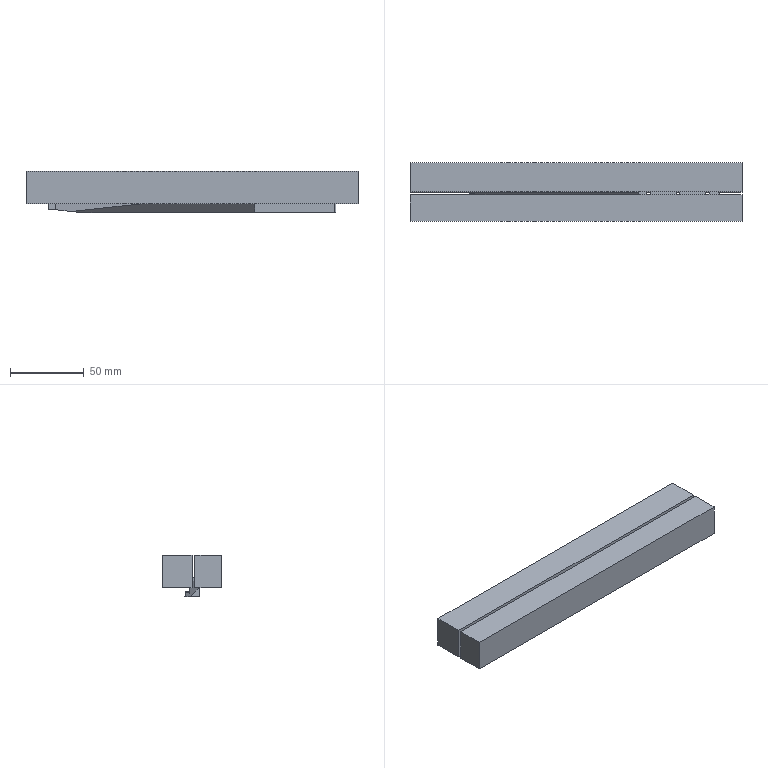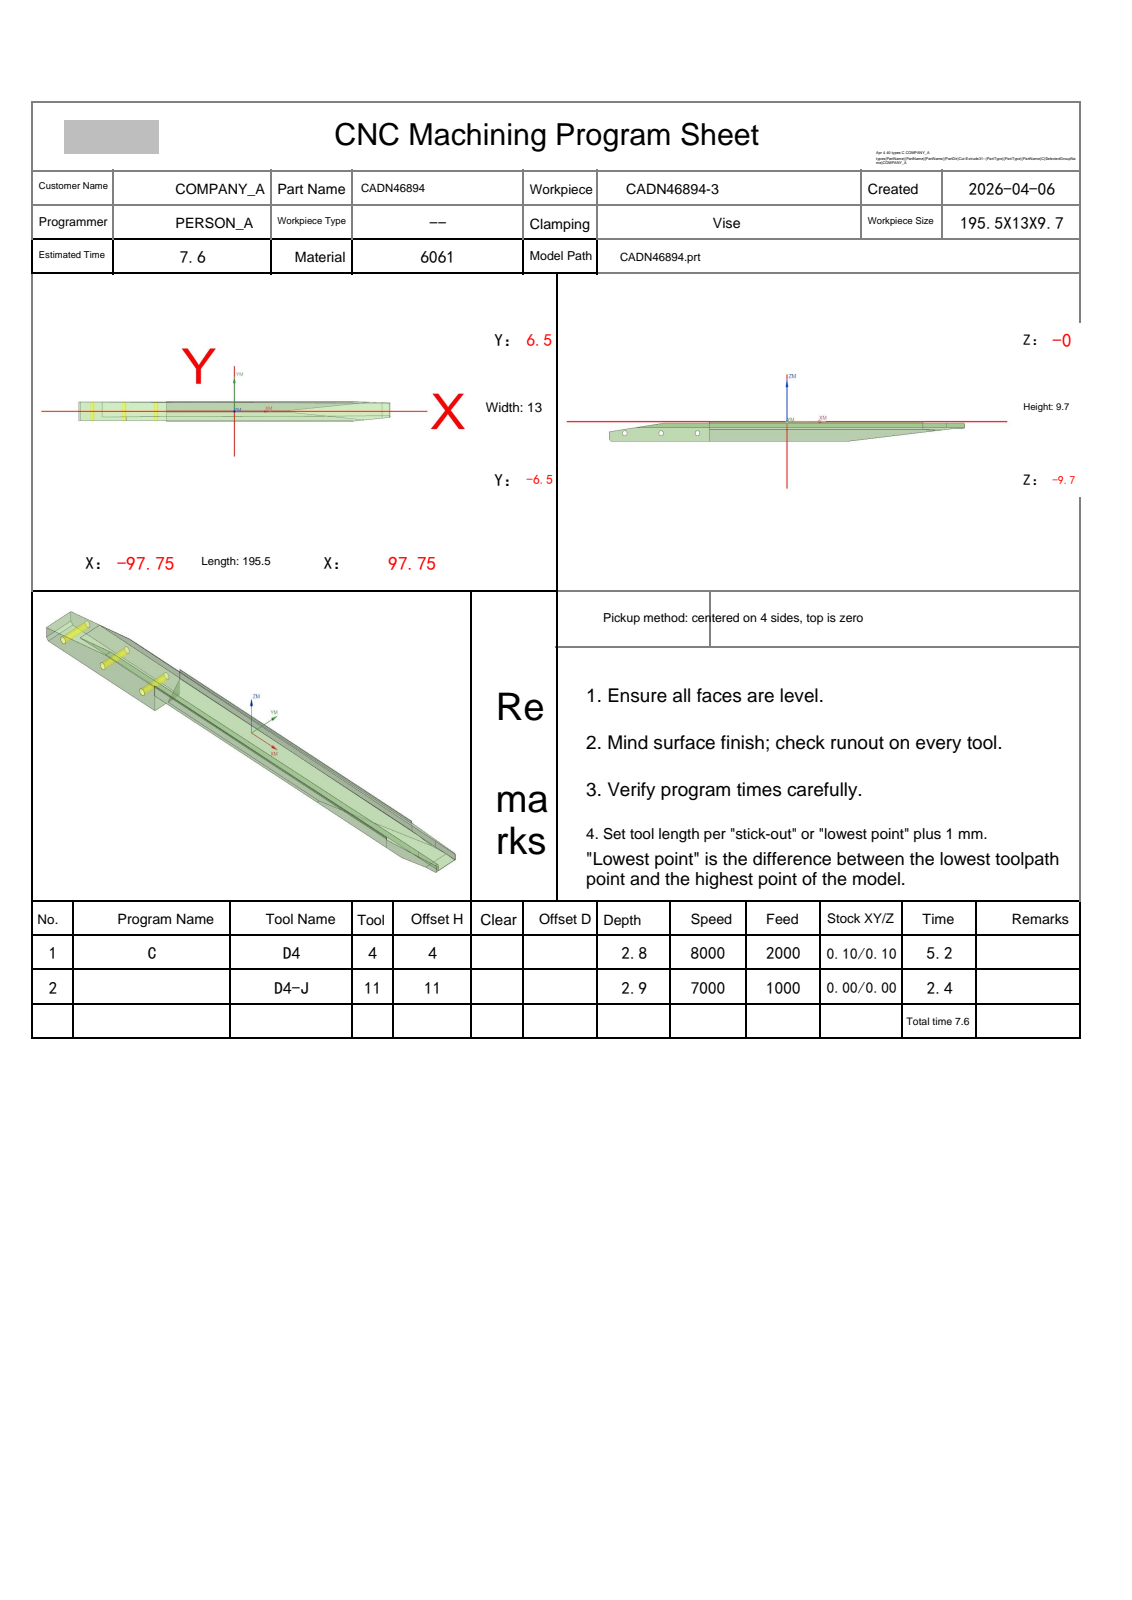NC program | NX | posted by the shop | part box 225.5 x 39.7 x 28 mm
Lines 1 to 1334 of 20119:
%
O0001
(Machine time: 20.00 MIN)
(===Total Tool:4===)
(T4=D4      D=4.   R=0.   D-  H04 Z=-12.35)
(T17=D2-J   D=2.   R=0.   D-  H17 Z=-12.4 )
(T19=D1.5-J D=1.5  R=0.   D-  H19 Z=-12.4 )
(T2=D6 chamfer tool   D=6.   R=0.   D-  H02 Z=-7.2  )
G80 G90 G17 G49 G40
G91 G28 Z0
M01
N1 T04 M06
(D4  D=4. R=0. H=04 ce=0.05 di=0.05)
G00 G90 G54 X-83.137 Y-4.487 M03 S8000
G43 H04 Z44.
M08
Z-5.5
G01 X-109.809 Y-4.336 Z-6.199 F2000.
X-142.722 Y-4.15
X-163.733 Y-4.85
X-163.768
G02 X-165.219 Y-4.641 I0.0 J5.15
X-166.626 Y-5.054 I-2.137 J4.685
G01 X-170.088 Y-5.55
X-65.732
G02 X-64.212 Y-5.779 I0.0 J-5.15
X-62.726 Y-5.387 I2.042 J-4.728
G01 X-55.848 Y-4.641
X-53.937 Y-4.05
X-49.469
X-53.851 Y-4.525
G03 X-53.937 Y-4.05 I-1.997 J-.116
G01 X-55.848 Y-4.641
X-109.809 Y-4.336
X-109.796 Y-2.05
X-142.751
X-143.451 Y-2.75
X-163.768
G02 X-165.387 Y-2.285 I0.0 J3.05
X-166.924 Y-2.975 I-1.969 J2.329
G01 X-193.45 Y-6.777
Y-7.725
G02 X-192.5 Y-7.65 I.95 J-5.975
G01 X-65.732
G02 X-64.085 Y-8.133 I0.0 J-3.05
X-62.499 Y-7.475 I1.915 J-2.374
G01 X-37.837 Y-4.8
X-21.345
X-21.441 Y-3.021
X-18.939 Y-2.75
X-20.049
X-20.749 Y-2.05
X-109.796
X-110.296
Z-5.699
G00 Z-5.5
X-83.137 Y-4.487
Z-5.699
G01 X-109.809 Y-4.336 Z-6.397
X-142.722 Y-4.15
X-163.733 Y-4.85
X-163.768
G02 X-165.219 Y-4.641 I0.0 J5.15
X-166.626 Y-5.054 I-2.137 J4.685
G01 X-170.088 Y-5.55
X-65.732
G02 X-64.212 Y-5.779 I0.0 J-5.15
X-62.726 Y-5.387 I2.042 J-4.728
G01 X-55.848 Y-4.641
X-53.937 Y-4.05
X-49.469
X-53.851 Y-4.525
G03 X-53.937 Y-4.05 I-1.997 J-.116
G01 X-55.848 Y-4.641
X-109.809 Y-4.336
X-109.796 Y-2.05
X-142.751
X-143.451 Y-2.75
X-163.768
G02 X-165.387 Y-2.285 I0.0 J3.05
X-166.924 Y-2.975 I-1.969 J2.329
G01 X-193.45 Y-6.777
Y-7.725
G02 X-192.5 Y-7.65 I.95 J-5.975
G01 X-65.732
G02 X-64.085 Y-8.133 I0.0 J-3.05
X-62.499 Y-7.475 I1.915 J-2.374
G01 X-37.837 Y-4.8
X-21.345
X-21.441 Y-3.021
X-18.939 Y-2.75
X-20.049
X-20.749 Y-2.05
X-109.796
X-110.296
Z-5.897
G00 Z-5.699
X-83.137 Y-4.487
Z-5.897
G01 X-109.809 Y-4.336 Z-6.595
X-142.722 Y-4.15
X-163.733 Y-4.85
X-163.768
G02 X-165.219 Y-4.641 I0.0 J5.15
X-166.626 Y-5.054 I-2.137 J4.685
G01 X-170.088 Y-5.55
X-65.732
G02 X-64.212 Y-5.779 I0.0 J-5.15
X-62.726 Y-5.387 I2.042 J-4.728
G01 X-55.848 Y-4.641
X-53.937 Y-4.05
X-49.469
X-53.851 Y-4.525
G03 X-53.937 Y-4.05 I-1.997 J-.116
G01 X-55.848 Y-4.641
X-109.809 Y-4.336
X-109.796 Y-2.05
X-142.751
X-143.451 Y-2.75
X-163.768
G02 X-165.387 Y-2.285 I0.0 J3.05
X-166.924 Y-2.975 I-1.969 J2.329
G01 X-193.45 Y-6.777
Y-7.725
G02 X-192.5 Y-7.65 I.95 J-5.975
G01 X-65.732
G02 X-64.085 Y-8.133 I0.0 J-3.05
X-62.499 Y-7.475 I1.915 J-2.374
G01 X-37.837 Y-4.8
X-21.345
X-21.441 Y-3.021
X-18.939 Y-2.75
X-20.049
X-20.749 Y-2.05
X-109.796
X-110.296
Z-6.095
G00 Z-5.897
X-83.137 Y-4.487
Z-6.095
G01 X-109.809 Y-4.336 Z-6.794
X-142.722 Y-4.15
X-163.733 Y-4.85
X-163.768
G02 X-165.219 Y-4.641 I0.0 J5.15
X-166.626 Y-5.054 I-2.137 J4.685
G01 X-170.088 Y-5.55
X-65.732
G02 X-64.212 Y-5.779 I0.0 J-5.15
X-62.726 Y-5.387 I2.042 J-4.728
G01 X-55.848 Y-4.641
X-53.937 Y-4.05
X-49.469
X-53.851 Y-4.525
G03 X-53.937 Y-4.05 I-1.997 J-.116
G01 X-55.848 Y-4.641
X-109.809 Y-4.336
X-109.796 Y-2.05
X-142.751
X-143.451 Y-2.75
X-163.768
G02 X-165.387 Y-2.285 I0.0 J3.05
X-166.924 Y-2.975 I-1.969 J2.329
G01 X-193.45 Y-6.777
Y-7.725
G02 X-192.5 Y-7.65 I.95 J-5.975
G01 X-65.732
G02 X-64.085 Y-8.133 I0.0 J-3.05
X-62.499 Y-7.475 I1.915 J-2.374
G01 X-37.837 Y-4.8
X-21.345
X-21.441 Y-3.021
X-18.939 Y-2.75
X-20.049
X-20.749 Y-2.05
X-109.796
X-110.296
Z-6.294
G00 Z-6.095
X-83.137 Y-4.487
Z-6.294
G01 X-109.809 Y-4.336 Z-6.992
X-142.722 Y-4.15
X-163.733 Y-4.85
X-163.768
G02 X-165.219 Y-4.641 I0.0 J5.15
X-166.626 Y-5.054 I-2.137 J4.685
G01 X-170.088 Y-5.55
X-65.732
G02 X-64.212 Y-5.779 I0.0 J-5.15
X-62.726 Y-5.387 I2.042 J-4.728
G01 X-55.848 Y-4.641
X-53.937 Y-4.05
X-49.469
X-53.851 Y-4.525
G03 X-53.937 Y-4.05 I-1.997 J-.116
G01 X-55.848 Y-4.641
X-109.809 Y-4.336
X-109.796 Y-2.05
X-142.751
X-143.451 Y-2.75
X-163.768
G02 X-165.387 Y-2.285 I0.0 J3.05
X-166.924 Y-2.975 I-1.969 J2.329
G01 X-193.45 Y-6.777
Y-7.725
G02 X-192.5 Y-7.65 I.95 J-5.975
G01 X-65.732
G02 X-64.085 Y-8.133 I0.0 J-3.05
X-62.499 Y-7.475 I1.915 J-2.374
G01 X-37.837 Y-4.8
X-21.345
X-21.441 Y-3.021
X-18.939 Y-2.75
X-20.049
X-20.749 Y-2.05
X-109.796
X-110.296
Z-6.492
G00 Z-6.294
X-83.137 Y-4.487
Z-6.492
G01 X-109.809 Y-4.336 Z-7.191
X-142.722 Y-4.15
X-163.733 Y-4.85
X-163.768
G02 X-165.219 Y-4.641 I0.0 J5.15
X-166.626 Y-5.054 I-2.137 J4.685
G01 X-170.088 Y-5.55
X-65.732
G02 X-64.212 Y-5.779 I0.0 J-5.15
X-62.726 Y-5.387 I2.042 J-4.728
G01 X-55.848 Y-4.641
X-53.937 Y-4.05
X-49.469
X-53.851 Y-4.525
G03 X-53.937 Y-4.05 I-1.997 J-.116
G01 X-55.848 Y-4.641
X-109.809 Y-4.336
X-109.796 Y-2.05
X-142.751
X-143.451 Y-2.75
X-163.768
G02 X-165.387 Y-2.285 I0.0 J3.05
X-166.924 Y-2.975 I-1.969 J2.329
G01 X-193.45 Y-6.777
Y-7.725
G02 X-192.5 Y-7.65 I.95 J-5.975
G01 X-65.732
G02 X-64.085 Y-8.133 I0.0 J-3.05
X-62.499 Y-7.475 I1.915 J-2.374
G01 X-37.837 Y-4.8
X-21.345
X-21.441 Y-3.021
X-18.939 Y-2.75
X-20.049
X-20.749 Y-2.05
X-109.796
X-110.296
Z-6.691
G00 Z-6.492
X-83.137 Y-4.487
Z-6.691
G01 X-109.809 Y-4.336 Z-7.389
X-142.722 Y-4.15
X-163.733 Y-4.85
X-163.768
G02 X-165.219 Y-4.641 I0.0 J5.15
X-166.626 Y-5.054 I-2.137 J4.685
G01 X-170.088 Y-5.55
X-65.732
G02 X-64.212 Y-5.779 I0.0 J-5.15
X-62.726 Y-5.387 I2.042 J-4.728
G01 X-55.848 Y-4.641
X-53.937 Y-4.05
X-49.469
X-53.851 Y-4.525
G03 X-53.937 Y-4.05 I-1.997 J-.116
G01 X-55.848 Y-4.641
X-109.809 Y-4.336
X-109.796 Y-2.05
X-142.751
X-143.451 Y-2.75
X-163.768
G02 X-165.387 Y-2.285 I0.0 J3.05
X-166.924 Y-2.975 I-1.969 J2.329
G01 X-193.45 Y-6.777
Y-7.725
G02 X-192.5 Y-7.65 I.95 J-5.975
G01 X-65.732
G02 X-64.085 Y-8.133 I0.0 J-3.05
X-62.499 Y-7.475 I1.915 J-2.374
G01 X-37.837 Y-4.8
X-21.345
X-21.441 Y-3.021
X-18.939 Y-2.75
X-20.049
X-20.749 Y-2.05
X-109.796
X-110.296
Z-6.889
G00 Z-6.691
X-83.137 Y-4.487
Z-6.889
G01 X-109.809 Y-4.336 Z-7.588
X-142.722 Y-4.15
X-163.733 Y-4.85
X-163.768
G02 X-165.219 Y-4.641 I0.0 J5.15
X-166.626 Y-5.054 I-2.137 J4.685
G01 X-170.088 Y-5.55
X-65.732
G02 X-64.212 Y-5.779 I0.0 J-5.15
X-62.726 Y-5.387 I2.042 J-4.728
G01 X-55.848 Y-4.641
X-53.937 Y-4.05
X-49.469
X-53.851 Y-4.525
G03 X-53.937 Y-4.05 I-1.997 J-.116
G01 X-55.848 Y-4.641
X-109.809 Y-4.336
X-109.796 Y-2.05
X-142.751
X-143.451 Y-2.75
X-163.768
G02 X-165.387 Y-2.285 I0.0 J3.05
X-166.924 Y-2.975 I-1.969 J2.329
G01 X-193.45 Y-6.777
Y-7.725
G02 X-192.5 Y-7.65 I.95 J-5.975
G01 X-65.732
G02 X-64.085 Y-8.133 I0.0 J-3.05
X-62.499 Y-7.475 I1.915 J-2.374
G01 X-37.837 Y-4.8
X-21.345
X-21.441 Y-3.021
X-18.939 Y-2.75
X-20.049
X-20.749 Y-2.05
X-109.796
X-110.296
Z-7.088
G00 Z-6.889
X-83.137 Y-4.487
Z-7.088
G01 X-109.809 Y-4.336 Z-7.786
X-142.722 Y-4.15
X-163.733 Y-4.85
X-163.768
G02 X-165.219 Y-4.641 I0.0 J5.15
X-166.626 Y-5.054 I-2.137 J4.685
G01 X-170.088 Y-5.55
X-65.732
G02 X-64.212 Y-5.779 I0.0 J-5.15
X-62.726 Y-5.387 I2.042 J-4.728
G01 X-55.848 Y-4.641
X-53.937 Y-4.05
X-49.469
X-53.851 Y-4.525
G03 X-53.937 Y-4.05 I-1.997 J-.116
G01 X-55.848 Y-4.641
X-109.809 Y-4.336
X-109.796 Y-2.05
X-142.751
X-143.451 Y-2.75
X-163.768
G02 X-165.387 Y-2.285 I0.0 J3.05
X-166.924 Y-2.975 I-1.969 J2.329
G01 X-193.45 Y-6.777
Y-7.725
G02 X-192.5 Y-7.65 I.95 J-5.975
G01 X-65.732
G02 X-64.085 Y-8.133 I0.0 J-3.05
X-62.499 Y-7.475 I1.915 J-2.374
G01 X-37.837 Y-4.8
X-21.345
X-21.441 Y-3.021
X-18.939 Y-2.75
X-20.049
X-20.749 Y-2.05
X-109.796
X-110.296
Z-7.286
G00 Z-7.088
X-83.137 Y-4.487
Z-7.286
G01 X-109.809 Y-4.336 Z-7.984
X-142.722 Y-4.15
X-163.733 Y-4.85
X-163.768
G02 X-165.219 Y-4.641 I0.0 J5.15
X-166.626 Y-5.054 I-2.137 J4.685
G01 X-170.088 Y-5.55
X-65.732
G02 X-64.212 Y-5.779 I0.0 J-5.15
X-62.726 Y-5.387 I2.042 J-4.728
G01 X-55.848 Y-4.641
X-53.937 Y-4.05
X-49.469
X-53.851 Y-4.525
G03 X-53.937 Y-4.05 I-1.997 J-.116
G01 X-55.848 Y-4.641
X-109.809 Y-4.336
X-109.796 Y-2.05
X-142.751
X-143.451 Y-2.75
X-163.768
G02 X-165.387 Y-2.285 I0.0 J3.05
X-166.924 Y-2.975 I-1.969 J2.329
G01 X-193.45 Y-6.777
Y-7.725
G02 X-192.5 Y-7.65 I.95 J-5.975
G01 X-65.732
G02 X-64.085 Y-8.133 I0.0 J-3.05
X-62.499 Y-7.475 I1.915 J-2.374
G01 X-37.837 Y-4.8
X-21.345
X-21.441 Y-3.021
X-18.939 Y-2.75
X-20.049
X-20.749 Y-2.05
X-109.796
X-110.296
Z-7.484
G00 Z-7.286
X-83.137 Y-4.487
Z-7.484
G01 X-109.809 Y-4.336 Z-8.183
X-142.722 Y-4.15
X-163.733 Y-4.85
X-163.768
G02 X-165.219 Y-4.641 I0.0 J5.15
X-166.626 Y-5.054 I-2.137 J4.685
G01 X-170.088 Y-5.55
X-65.732
G02 X-64.212 Y-5.779 I0.0 J-5.15
X-62.726 Y-5.387 I2.042 J-4.728
G01 X-55.848 Y-4.641
X-53.937 Y-4.05
X-49.469
X-53.851 Y-4.525
G03 X-53.937 Y-4.05 I-1.997 J-.116
G01 X-55.848 Y-4.641
X-109.809 Y-4.336
X-109.796 Y-2.05
X-142.751
X-143.451 Y-2.75
X-163.768
G02 X-165.387 Y-2.285 I0.0 J3.05
X-166.924 Y-2.975 I-1.969 J2.329
G01 X-193.45 Y-6.777
Y-7.725
G02 X-192.5 Y-7.65 I.95 J-5.975
G01 X-65.732
G02 X-64.085 Y-8.133 I0.0 J-3.05
X-62.499 Y-7.475 I1.915 J-2.374
G01 X-37.837 Y-4.8
X-21.345
X-21.441 Y-3.021
X-18.939 Y-2.75
X-20.049
X-20.749 Y-2.05
X-109.796
X-110.296
Z-7.683
G00 Z-7.484
X-83.137 Y-4.487
Z-7.683
G01 X-109.809 Y-4.336 Z-8.381
X-142.722 Y-4.15
X-163.733 Y-4.85
X-163.768
G02 X-165.219 Y-4.641 I0.0 J5.15
X-166.626 Y-5.054 I-2.137 J4.685
G01 X-170.088 Y-5.55
X-65.732
G02 X-64.212 Y-5.779 I0.0 J-5.15
X-62.726 Y-5.387 I2.042 J-4.728
G01 X-55.848 Y-4.641
X-53.937 Y-4.05
X-49.469
X-53.851 Y-4.525
G03 X-53.937 Y-4.05 I-1.997 J-.116
G01 X-55.848 Y-4.641
X-109.809 Y-4.336
X-109.796 Y-2.05
X-142.751
X-143.451 Y-2.75
X-163.768
G02 X-165.387 Y-2.285 I0.0 J3.05
X-166.924 Y-2.975 I-1.969 J2.329
G01 X-193.45 Y-6.777
Y-7.725
G02 X-192.5 Y-7.65 I.95 J-5.975
G01 X-65.732
G02 X-64.085 Y-8.133 I0.0 J-3.05
X-62.499 Y-7.475 I1.915 J-2.374
G01 X-37.837 Y-4.8
X-21.345
X-21.441 Y-3.021
X-18.939 Y-2.75
X-20.049
X-20.749 Y-2.05
X-109.796
X-110.296
Z-7.881
G00 Z-7.683
X-83.137 Y-4.487
Z-7.881
G01 X-109.809 Y-4.336 Z-8.58
X-142.722 Y-4.15
X-163.733 Y-4.85
X-163.768
G02 X-165.219 Y-4.641 I0.0 J5.15
X-166.626 Y-5.054 I-2.137 J4.685
G01 X-170.088 Y-5.55
X-65.732
G02 X-64.212 Y-5.779 I0.0 J-5.15
X-62.726 Y-5.387 I2.042 J-4.728
G01 X-55.848 Y-4.641
X-53.937 Y-4.05
X-49.469
X-53.851 Y-4.525
G03 X-53.937 Y-4.05 I-1.997 J-.116
G01 X-55.848 Y-4.641
X-109.809 Y-4.336
X-109.796 Y-2.05
X-142.751
X-143.451 Y-2.75
X-163.768
G02 X-165.387 Y-2.285 I0.0 J3.05
X-166.924 Y-2.975 I-1.969 J2.329
G01 X-193.45 Y-6.777
Y-7.725
G02 X-192.5 Y-7.65 I.95 J-5.975
G01 X-65.732
G02 X-64.085 Y-8.133 I0.0 J-3.05
X-62.499 Y-7.475 I1.915 J-2.374
G01 X-37.837 Y-4.8
X-21.345
X-21.441 Y-3.021
X-18.939 Y-2.75
X-20.049
X-20.749 Y-2.05
X-109.796
X-110.296
Z-8.08
G00 Z-7.881
X-83.137 Y-4.487
Z-8.08
G01 X-109.809 Y-4.336 Z-8.778
X-142.722 Y-4.15
X-163.733 Y-4.85
X-163.768
G02 X-165.219 Y-4.641 I0.0 J5.15
X-166.626 Y-5.054 I-2.137 J4.685
G01 X-170.088 Y-5.55
X-65.732
G02 X-64.212 Y-5.779 I0.0 J-5.15
X-62.726 Y-5.387 I2.042 J-4.728
G01 X-55.848 Y-4.641
X-53.937 Y-4.05
X-49.469
X-53.851 Y-4.525
G03 X-53.937 Y-4.05 I-1.997 J-.116
G01 X-55.848 Y-4.641
X-109.809 Y-4.336
X-109.796 Y-2.05
X-142.751
X-143.451 Y-2.75
X-163.768
G02 X-165.387 Y-2.285 I0.0 J3.05
X-166.924 Y-2.975 I-1.969 J2.329
G01 X-193.45 Y-6.777
Y-7.725
G02 X-192.5 Y-7.65 I.95 J-5.975
G01 X-65.732
G02 X-64.085 Y-8.133 I0.0 J-3.05
X-62.499 Y-7.475 I1.915 J-2.374
G01 X-37.837 Y-4.8
X-21.345
X-21.441 Y-3.021
X-18.939 Y-2.75
X-20.049
X-20.749 Y-2.05
X-109.796
X-110.296
Z-8.278
G00 Z-8.08
X-83.137 Y-4.487
Z-8.278
G01 X-109.809 Y-4.336 Z-8.977
X-142.722 Y-4.15
X-163.733 Y-4.85
X-163.768
G02 X-165.219 Y-4.641 I0.0 J5.15
X-166.626 Y-5.054 I-2.137 J4.685
G01 X-170.088 Y-5.55
X-65.732
G02 X-64.212 Y-5.779 I0.0 J-5.15
X-62.726 Y-5.387 I2.042 J-4.728
G01 X-55.848 Y-4.641
X-53.937 Y-4.05
X-49.469
X-53.851 Y-4.525
G03 X-53.937 Y-4.05 I-1.997 J-.116
G01 X-55.848 Y-4.641
X-109.809 Y-4.336
X-109.796 Y-2.05
X-142.751
X-143.451 Y-2.75
X-163.768
G02 X-165.387 Y-2.285 I0.0 J3.05
X-166.924 Y-2.975 I-1.969 J2.329
G01 X-193.45 Y-6.777
Y-7.725
G02 X-192.5 Y-7.65 I.95 J-5.975
G01 X-65.732
G02 X-64.085 Y-8.133 I0.0 J-3.05
X-62.499 Y-7.475 I1.915 J-2.374
G01 X-37.837 Y-4.8
X-21.345
X-21.441 Y-3.021
X-18.939 Y-2.75
X-20.049
X-20.749 Y-2.05
X-109.796
X-110.296
Z-8.477
G00 Z-8.278
X-83.137 Y-4.487
Z-8.477
G01 X-109.809 Y-4.336 Z-9.175
X-142.722 Y-4.15
X-163.733 Y-4.85
X-163.768
G02 X-165.219 Y-4.641 I0.0 J5.15
X-166.626 Y-5.054 I-2.137 J4.685
G01 X-170.088 Y-5.55
X-65.732
G02 X-64.212 Y-5.779 I0.0 J-5.15
X-62.726 Y-5.387 I2.042 J-4.728
G01 X-55.848 Y-4.641
X-53.937 Y-4.05
X-49.469
X-53.851 Y-4.525
G03 X-53.937 Y-4.05 I-1.997 J-.116
G01 X-55.848 Y-4.641
X-109.809 Y-4.336
X-109.796 Y-2.05
X-142.751
X-143.451 Y-2.75
X-163.768
G02 X-165.387 Y-2.285 I0.0 J3.05
X-166.924 Y-2.975 I-1.969 J2.329
G01 X-193.45 Y-6.777
Y-7.725
G02 X-192.5 Y-7.65 I.95 J-5.975
G01 X-65.732
G02 X-64.085 Y-8.133 I0.0 J-3.05
X-62.499 Y-7.475 I1.915 J-2.374
G01 X-37.837 Y-4.8
X-21.345
X-21.441 Y-3.021
X-18.939 Y-2.75
X-20.049
X-20.749 Y-2.05
X-109.796
X-110.296
Z-8.675
G00 Z-8.477
X-83.137 Y-4.487
Z-8.675
G01 X-109.809 Y-4.336 Z-9.373
X-142.722 Y-4.15
X-163.733 Y-4.85
X-163.768
G02 X-165.219 Y-4.641 I0.0 J5.15
X-166.626 Y-5.054 I-2.137 J4.685
G01 X-170.088 Y-5.55
X-65.732
G02 X-64.212 Y-5.779 I0.0 J-5.15
X-62.726 Y-5.387 I2.042 J-4.728
G01 X-55.848 Y-4.641
X-53.937 Y-4.05
X-49.469
X-53.851 Y-4.525
G03 X-53.937 Y-4.05 I-1.997 J-.116
G01 X-55.848 Y-4.641
X-109.809 Y-4.336
X-109.796 Y-2.05
X-142.751
X-143.451 Y-2.75
X-163.768
G02 X-165.387 Y-2.285 I0.0 J3.05
X-166.924 Y-2.975 I-1.969 J2.329
G01 X-193.45 Y-6.777
Y-7.725
G02 X-192.5 Y-7.65 I.95 J-5.975
G01 X-65.732
G02 X-64.085 Y-8.133 I0.0 J-3.05
X-62.499 Y-7.475 I1.915 J-2.374
G01 X-37.837 Y-4.8
X-21.345
X-21.441 Y-3.021
X-18.939 Y-2.75
X-20.049
X-20.749 Y-2.05
X-109.796
X-110.296
Z-8.873
G00 Z-8.675
X-83.137 Y-4.487
Z-8.873
G01 X-109.809 Y-4.336 Z-9.572
X-142.722 Y-4.15
X-163.733 Y-4.85
X-163.768
G02 X-165.219 Y-4.641 I0.0 J5.15
X-166.626 Y-5.054 I-2.137 J4.685
G01 X-170.088 Y-5.55
X-65.732
G02 X-64.212 Y-5.779 I0.0 J-5.15
X-62.726 Y-5.387 I2.042 J-4.728
G01 X-55.848 Y-4.641
X-53.937 Y-4.05
X-49.469
X-53.851 Y-4.525
G03 X-53.937 Y-4.05 I-1.997 J-.116
G01 X-55.848 Y-4.641
X-109.809 Y-4.336
X-109.796 Y-2.05
X-142.751
X-143.451 Y-2.75
X-163.768
G02 X-165.387 Y-2.285 I0.0 J3.05
X-166.924 Y-2.975 I-1.969 J2.329
G01 X-193.45 Y-6.777
Y-7.725
G02 X-192.5 Y-7.65 I.95 J-5.975
G01 X-65.732
G02 X-64.085 Y-8.133 I0.0 J-3.05
X-62.499 Y-7.475 I1.915 J-2.374
G01 X-37.837 Y-4.8
X-21.345
X-21.441 Y-3.021
X-18.939 Y-2.75
X-20.049
X-20.749 Y-2.05
X-109.796
X-110.296
Z-9.072
G00 Z-8.873
X-83.137 Y-4.487
Z-9.072
G01 X-109.809 Y-4.336 Z-9.77
X-142.722 Y-4.15
X-163.733 Y-4.85
X-163.768
G02 X-165.219 Y-4.641 I0.0 J5.15
X-166.626 Y-5.054 I-2.137 J4.685
G01 X-170.088 Y-5.55
X-65.732
G02 X-64.212 Y-5.779 I0.0 J-5.15
X-62.726 Y-5.387 I2.042 J-4.728
G01 X-55.848 Y-4.641
X-53.937 Y-4.05
X-49.469
X-53.851 Y-4.525
G03 X-53.937 Y-4.05 I-1.997 J-.116
G01 X-55.848 Y-4.641
X-109.809 Y-4.336
X-109.796 Y-2.05
X-142.751
X-143.451 Y-2.75
X-163.768
G02 X-165.387 Y-2.285 I0.0 J3.05
X-166.924 Y-2.975 I-1.969 J2.329
G01 X-193.45 Y-6.777
Y-7.725
G02 X-192.5 Y-7.65 I.95 J-5.975
G01 X-65.732
G02 X-64.085 Y-8.133 I0.0 J-3.05
X-62.499 Y-7.475 I1.915 J-2.374
G01 X-37.837 Y-4.8
X-21.345
X-21.441 Y-3.021
X-18.939 Y-2.75
X-20.049
X-20.749 Y-2.05
X-109.796
X-110.296
Z-9.27
G00 Z-9.072
X-83.137 Y-4.487
Z-9.27
G01 X-109.809 Y-4.336 Z-9.969
X-142.722 Y-4.15
X-163.733 Y-4.85
X-163.768
G02 X-165.219 Y-4.641 I0.0 J5.15
X-166.626 Y-5.054 I-2.137 J4.685
G01 X-170.088 Y-5.55
X-65.732
G02 X-64.212 Y-5.779 I0.0 J-5.15
X-62.726 Y-5.387 I2.042 J-4.728
G01 X-55.848 Y-4.641
X-53.937 Y-4.05
X-49.469
X-53.851 Y-4.525
G03 X-53.937 Y-4.05 I-1.997 J-.116
G01 X-55.848 Y-4.641
X-109.809 Y-4.336
X-109.796 Y-2.05
X-142.751
X-143.451 Y-2.75
X-163.768
G02 X-165.387 Y-2.285 I0.0 J3.05
X-166.924 Y-2.975 I-1.969 J2.329
G01 X-193.45 Y-6.777
Y-7.725
G02 X-192.5 Y-7.65 I.95 J-5.975
G01 X-65.732
G02 X-64.085 Y-8.133 I0.0 J-3.05
X-62.499 Y-7.475 I1.915 J-2.374
G01 X-37.837 Y-4.8
X-21.345
X-21.441 Y-3.021
X-18.939 Y-2.75
X-20.049
X-20.749 Y-2.05
X-109.796
X-110.296
Z-9.469
G00 Z-9.27
X-83.137 Y-4.487
Z-9.469
G01 X-109.809 Y-4.336 Z-10.167
X-142.722 Y-4.15
X-163.733 Y-4.85
X-163.768
G02 X-165.219 Y-4.641 I0.0 J5.15
X-166.626 Y-5.054 I-2.137 J4.685
G01 X-170.088 Y-5.55
X-65.732
G02 X-64.212 Y-5.779 I0.0 J-5.15
X-62.726 Y-5.387 I2.042 J-4.728
G01 X-55.848 Y-4.641
X-53.937 Y-4.05
X-49.469
X-53.851 Y-4.525
G03 X-53.937 Y-4.05 I-1.997 J-.116
G01 X-55.848 Y-4.641
X-109.809 Y-4.336
X-109.796 Y-2.05
X-142.751
X-143.451 Y-2.75
X-163.768
G02 X-165.387 Y-2.285 I0.0 J3.05
X-166.924 Y-2.975 I-1.969 J2.329
G01 X-193.45 Y-6.777
Y-7.725
G02 X-192.5 Y-7.65 I.95 J-5.975
G01 X-65.732
G02 X-64.085 Y-8.133 I0.0 J-3.05
X-62.499 Y-7.475 I1.915 J-2.374
G01 X-37.837 Y-4.8
X-21.345
X-21.441 Y-3.021
X-18.939 Y-2.75
X-20.049
X-20.749 Y-2.05
X-109.796
X-110.296
Z-9.667
G00 Z-9.469
X-83.137 Y-4.487
Z-9.667
G01 X-109.809 Y-4.336 Z-10.366
X-142.722 Y-4.15
X-163.733 Y-4.85
X-163.768
G02 X-165.219 Y-4.641 I0.0 J5.15
X-166.626 Y-5.054 I-2.137 J4.685
G01 X-170.088 Y-5.55
X-65.732
G02 X-64.212 Y-5.779 I0.0 J-5.15
X-62.726 Y-5.387 I2.042 J-4.728
G01 X-55.848 Y-4.641
X-53.937 Y-4.05
X-49.469
X-53.851 Y-4.525
G03 X-53.937 Y-4.05 I-1.997 J-.116
G01 X-55.848 Y-4.641
X-109.809 Y-4.336
X-109.796 Y-2.05
X-142.751
X-143.451 Y-2.75
X-163.768
G02 X-165.387 Y-2.285 I0.0 J3.05
X-166.924 Y-2.975 I-1.969 J2.329
G01 X-193.45 Y-6.777
Y-7.725
G02 X-192.5 Y-7.65 I.95 J-5.975
G01 X-65.732
G02 X-64.085 Y-8.133 I0.0 J-3.05
X-62.499 Y-7.475 I1.915 J-2.374
G01 X-37.837 Y-4.8
X-21.345
X-21.441 Y-3.021
X-18.939 Y-2.75
X-20.049
X-20.749 Y-2.05
X-109.796
X-110.296
Z-9.866
G00 Z-9.667
X-83.137 Y-4.487
Z-9.866
G01 X-109.809 Y-4.336 Z-10.564
X-142.722 Y-4.15
X-163.733 Y-4.85
X-163.768
G02 X-165.219 Y-4.641 I0.0 J5.15
X-166.626 Y-5.054 I-2.137 J4.685
G01 X-170.088 Y-5.55
X-65.732
G02 X-64.212 Y-5.779 I0.0 J-5.15
X-62.726 Y-5.387 I2.042 J-4.728
G01 X-55.848 Y-4.641
X-53.937 Y-4.05
X-49.469
X-53.851 Y-4.525
G03 X-53.937 Y-4.05 I-1.997 J-.116
G01 X-55.848 Y-4.641
X-109.809 Y-4.336
X-109.796 Y-2.05
X-142.751
X-143.451 Y-2.75
X-163.768
G02 X-165.387 Y-2.285 I0.0 J3.05
X-166.924 Y-2.975 I-1.969 J2.329
G01 X-193.45 Y-6.777
Y-7.725
G02 X-192.5 Y-7.65 I.95 J-5.975
G01 X-65.732
G02 X-64.085 Y-8.133 I0.0 J-3.05
X-62.499 Y-7.475 I1.915 J-2.374
G01 X-37.837 Y-4.8
X-21.345
X-21.441 Y-3.021
X-18.939 Y-2.75
X-20.049
X-20.749 Y-2.05
X-109.796
X-110.296
Z-10.064
G00 Z-9.866
X-83.137 Y-4.487
Z-10.064
G01 X-109.809 Y-4.336 Z-10.763
X-142.722 Y-4.15
X-163.733 Y-4.85
X-163.768
G02 X-165.219 Y-4.641 I0.0 J5.15
X-166.626 Y-5.054 I-2.137 J4.685
G01 X-170.088 Y-5.55
X-65.732
G02 X-64.212 Y-5.779 I0.0 J-5.15
X-62.726 Y-5.387 I2.042 J-4.728
G01 X-55.848 Y-4.641
X-53.937 Y-4.05
X-49.469
X-53.851 Y-4.525
G03 X-53.937 Y-4.05 I-1.997 J-.116
G01 X-55.848 Y-4.641
X-109.809 Y-4.336
X-109.796 Y-2.05
X-142.751
X-143.451 Y-2.75
X-163.768
G02 X-165.387 Y-2.285 I0.0 J3.05
X-166.924 Y-2.975 I-1.969 J2.329
G01 X-193.45 Y-6.777
Y-7.725
G02 X-192.5 Y-7.65 I.95 J-5.975
G01 X-65.732
G02 X-64.085 Y-8.133 I0.0 J-3.05
X-62.499 Y-7.475 I1.915 J-2.374
G01 X-37.837 Y-4.8
X-21.345
X-21.441 Y-3.021
X-18.939 Y-2.75
X-20.049
X-20.749 Y-2.05
X-109.796
X-110.296
Z-10.263
G00 Z-10.064
X-83.137 Y-4.487
Z-10.263
G01 X-109.809 Y-4.336 Z-10.961
X-142.722 Y-4.15
X-163.733 Y-4.85
X-163.768
G02 X-165.219 Y-4.641 I0.0 J5.15
X-166.626 Y-5.054 I-2.137 J4.685
G01 X-170.088 Y-5.55
X-65.732
G02 X-64.212 Y-5.779 I0.0 J-5.15
X-62.726 Y-5.387 I2.042 J-4.728
G01 X-55.848 Y-4.641
X-53.937 Y-4.05
X-49.469
X-53.851 Y-4.525
G03 X-53.937 Y-4.05 I-1.997 J-.116
G01 X-55.848 Y-4.641
X-109.809 Y-4.336
X-109.796 Y-2.05
X-142.751
X-143.451 Y-2.75
X-163.768
G02 X-165.387 Y-2.285 I0.0 J3.05
X-166.924 Y-2.975 I-1.969 J2.329
G01 X-193.45 Y-6.777
Y-7.725
G02 X-192.5 Y-7.65 I.95 J-5.975
G01 X-65.732
G02 X-64.085 Y-8.133 I0.0 J-3.05
X-62.499 Y-7.475 I1.915 J-2.374
G01 X-37.837 Y-4.8
X-21.345
X-21.441 Y-3.021
X-18.939 Y-2.75
X-20.049
X-20.749 Y-2.05
X-109.796
X-110.296
Z-10.461
G00 Z-10.263
X-83.137 Y-4.487
Z-10.461
G01 X-109.809 Y-4.336 Z-11.159
X-142.722 Y-4.15
X-163.733 Y-4.85
X-163.768
G02 X-165.219 Y-4.641 I0.0 J5.15
X-166.626 Y-5.054 I-2.137 J4.685
G01 X-170.088 Y-5.55
X-65.732
G02 X-64.212 Y-5.779 I0.0 J-5.15
X-62.726 Y-5.387 I2.042 J-4.728
G01 X-55.848 Y-4.641
X-53.937 Y-4.05
X-49.469
X-53.851 Y-4.525
G03 X-53.937 Y-4.05 I-1.997 J-.116
G01 X-55.848 Y-4.641
X-109.809 Y-4.336
X-109.796 Y-2.05
X-142.751
X-143.451 Y-2.75
X-163.768
G02 X-165.387 Y-2.285 I0.0 J3.05
X-166.924 Y-2.975 I-1.969 J2.329
G01 X-193.45 Y-6.777
Y-7.725
G02 X-192.5 Y-7.65 I.95 J-5.975
G01 X-65.732
G02 X-64.085 Y-8.133 I0.0 J-3.05
X-62.499 Y-7.475 I1.915 J-2.374
G01 X-37.837 Y-4.8
X-21.345
X-21.441 Y-3.021
X-18.939 Y-2.75
X-20.049
X-20.749 Y-2.05
X-109.796
X-110.296
Z-10.659
G00 Z-10.461
X-83.137 Y-4.487
Z-10.659
G01 X-109.809 Y-4.336 Z-11.358
X-142.722 Y-4.15
X-163.733 Y-4.85
X-163.768
G02 X-165.219 Y-4.641 I0.0 J5.15
X-166.626 Y-5.054 I-2.137 J4.685
G01 X-170.088 Y-5.55
X-65.732
G02 X-64.212 Y-5.779 I0.0 J-5.15
X-62.726 Y-5.387 I2.042 J-4.728
G01 X-55.848 Y-4.641
X-53.937 Y-4.05
X-49.469
X-53.851 Y-4.525
G03 X-53.937 Y-4.05 I-1.997 J-.116
G01 X-55.848 Y-4.641
X-109.809 Y-4.336
X-109.796 Y-2.05
X-142.751
X-143.451 Y-2.75
X-163.768
G02 X-165.387 Y-2.285 I0.0 J3.05
X-166.924 Y-2.975 I-1.969 J2.329
G01 X-193.45 Y-6.777
Y-7.725
G02 X-192.5 Y-7.65 I.95 J-5.975
G01 X-65.732
G02 X-64.085 Y-8.133 I0.0 J-3.05
X-62.499 Y-7.475 I1.915 J-2.374
G01 X-37.837 Y-4.8
X-21.345
X-21.441 Y-3.021
X-18.939 Y-2.75
X-20.049
X-20.749 Y-2.05
X-109.796
X-110.296
Z-10.858
G00 Z-10.659
X-83.137 Y-4.487
Z-10.858
G01 X-109.809 Y-4.336 Z-11.556
X-142.722 Y-4.15
X-163.733 Y-4.85
X-163.768
G02 X-165.219 Y-4.641 I0.0 J5.15
X-166.626 Y-5.054 I-2.137 J4.685
G01 X-170.088 Y-5.55
X-65.732
G02 X-64.212 Y-5.779 I0.0 J-5.15
X-62.726 Y-5.387 I2.042 J-4.728
G01 X-55.848 Y-4.641
X-53.937 Y-4.05
X-49.469
X-53.851 Y-4.525
G03 X-53.937 Y-4.05 I-1.997 J-.116
G01 X-55.848 Y-4.641
X-109.809 Y-4.336
X-109.796 Y-2.05
X-142.751
X-143.451 Y-2.75
X-163.768
G02 X-165.387 Y-2.285 I0.0 J3.05
X-166.924 Y-2.975 I-1.969 J2.329
G01 X-193.45 Y-6.777
Y-7.725
G02 X-192.5 Y-7.65 I.95 J-5.975
G01 X-65.732
G02 X-64.085 Y-8.133 I0.0 J-3.05
X-62.499 Y-7.475 I1.915 J-2.374
G01 X-37.837 Y-4.8
X-21.345
X-21.441 Y-3.021
X-18.939 Y-2.75
X-20.049
X-20.749 Y-2.05
X-109.796
X-110.296
Z-11.056
G00 Z-10.858
X-83.137 Y-4.487
Z-11.056
G01 X-109.809 Y-4.336 Z-11.755
X-142.722 Y-4.15
X-163.733 Y-4.85
X-163.768
G02 X-165.219 Y-4.641 I0.0 J5.15
X-166.626 Y-5.054 I-2.137 J4.685
G01 X-170.088 Y-5.55
X-65.732
G02 X-64.212 Y-5.779 I0.0 J-5.15
X-62.726 Y-5.387 I2.042 J-4.728
G01 X-55.848 Y-4.641
X-53.937 Y-4.05
X-49.469
X-53.851 Y-4.525
G03 X-53.937 Y-4.05 I-1.997 J-.116
G01 X-55.848 Y-4.641
X-109.809 Y-4.336
X-109.796 Y-2.05
X-142.751
X-143.451 Y-2.75
X-163.768
G02 X-165.387 Y-2.285 I0.0 J3.05
X-166.924 Y-2.975 I-1.969 J2.329
G01 X-193.45 Y-6.777
Y-7.725
G02 X-192.5 Y-7.65 I.95 J-5.975
G01 X-65.732
G02 X-64.085 Y-8.133 I0.0 J-3.05
X-62.499 Y-7.475 I1.915 J-2.374
G01 X-37.837 Y-4.8
X-21.345
X-21.441 Y-3.021
X-18.939 Y-2.75
X-20.049
X-20.749 Y-2.05
X-109.796
X-110.296
Z-11.255
G00 Z-11.056
X-83.137 Y-4.487
Z-11.255
G01 X-109.809 Y-4.336 Z-11.953
X-142.722 Y-4.15
X-163.733 Y-4.85
X-163.768
G02 X-165.219 Y-4.641 I0.0 J5.15
X-166.626 Y-5.054 I-2.137 J4.685
G01 X-170.088 Y-5.55
X-65.732
G02 X-64.212 Y-5.779 I0.0 J-5.15
X-62.726 Y-5.387 I2.042 J-4.728
G01 X-55.848 Y-4.641
X-53.937 Y-4.05
X-49.469
X-53.851 Y-4.525
G03 X-53.937 Y-4.05 I-1.997 J-.116
G01 X-55.848 Y-4.641
X-109.809 Y-4.336
X-109.796 Y-2.05
X-142.751
X-143.451 Y-2.75
X-163.768
G02 X-165.387 Y-2.285 I0.0 J3.05
X-166.924 Y-2.975 I-1.969 J2.329
G01 X-193.45 Y-6.777
Y-7.725
G02 X-192.5 Y-7.65 I.95 J-5.975
G01 X-65.732
G02 X-64.085 Y-8.133 I0.0 J-3.05
X-62.499 Y-7.475 I1.915 J-2.374
G01 X-37.837 Y-4.8
X-21.345
X-21.441 Y-3.021
X-18.939 Y-2.75
X-20.049
X-20.749 Y-2.05
X-109.796
X-110.296
Z-11.453
G00 Z-11.255
X-83.137 Y-4.487
Z-11.453
G01 X-109.809 Y-4.336 Z-12.152
X-142.722 Y-4.15
X-163.733 Y-4.85
X-163.768
G02 X-165.219 Y-4.641 I0.0 J5.15
X-166.626 Y-5.054 I-2.137 J4.685
G01 X-170.088 Y-5.55
X-65.732
G02 X-64.212 Y-5.779 I0.0 J-5.15
X-62.726 Y-5.387 I2.042 J-4.728
G01 X-55.848 Y-4.641
X-53.937 Y-4.05
X-49.469
X-53.851 Y-4.525
G03 X-53.937 Y-4.05 I-1.997 J-.116
G01 X-55.848 Y-4.641
X-109.809 Y-4.336
X-109.796 Y-2.05
X-142.751
X-143.451 Y-2.75
X-163.768
G02 X-165.387 Y-2.285 I0.0 J3.05
X-166.924 Y-2.975 I-1.969 J2.329
G01 X-193.45 Y-6.777
Y-7.725
G02 X-192.5 Y-7.65 I.95 J-5.975
G01 X-65.732
G02 X-64.085 Y-8.133 I0.0 J-3.05
X-62.499 Y-7.475 I1.915 J-2.374
G01 X-37.837 Y-4.8
X-21.345
X-21.441 Y-3.021
X-18.939 Y-2.75
X-20.049
X-20.749 Y-2.05
X-109.796
X-110.296
Z-11.652
G00 Z-11.453
X-83.137 Y-4.487
Z-11.652
G01 X-109.809 Y-4.336 Z-12.35
X-142.722 Y-4.15
X-163.733 Y-4.85
X-163.768
G02 X-165.219 Y-4.641 I0.0 J5.15
X-166.626 Y-5.054 I-2.137 J4.685
G01 X-170.088 Y-5.55
X-65.732
G02 X-64.212 Y-5.779 I0.0 J-5.15
X-62.726 Y-5.387 I2.042 J-4.728
G01 X-55.848 Y-4.641
X-53.937 Y-4.05
X-49.469
X-53.851 Y-4.525
G03 X-53.937 Y-4.05 I-1.997 J-.116
G01 X-55.848 Y-4.641
X-109.809 Y-4.336
X-109.796 Y-2.05
X-142.751
X-143.451 Y-2.75
X-163.768
G02 X-165.387 Y-2.285 I0.0 J3.05
X-166.924 Y-2.975 I-1.969 J2.329
G01 X-193.45 Y-6.777
Y-7.725
G02 X-192.5 Y-7.65 I.95 J-5.975
G01 X-65.732
G02 X-64.085 Y-8.133 I0.0 J-3.05
X-62.499 Y-7.475 I1.915 J-2.374
G01 X-37.837 Y-4.8
X-21.345
X-21.441 Y-3.021
X-18.939 Y-2.75
X-20.049
X-20.749 Y-2.05
X-109.796
X-110.296
Z-11.85
G00 Z44.
G91 G28 Z0.0
M05
M09
G91 G28 Z0.0
M01